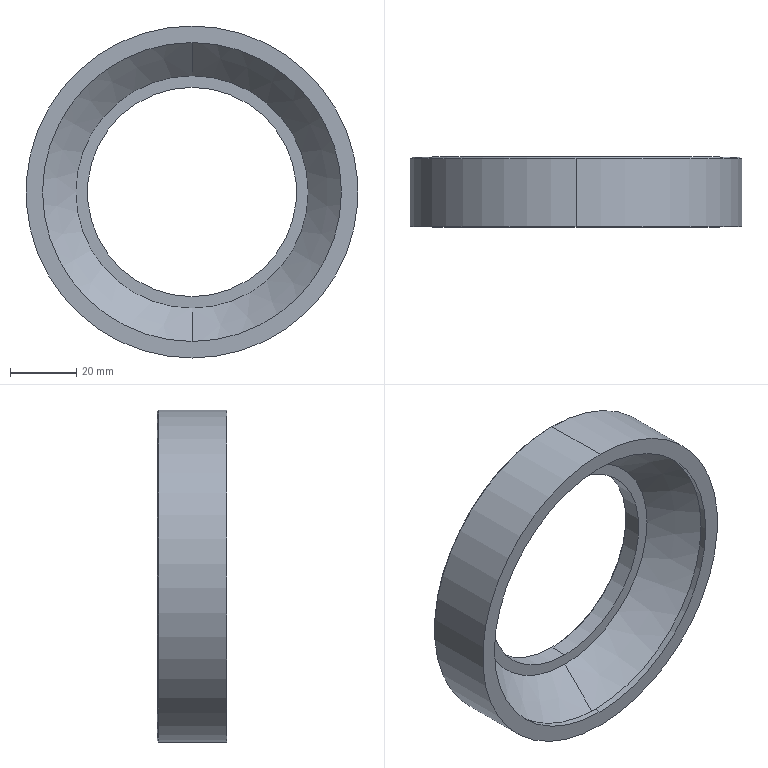Part | STEP file | WLDR-LA100-W light source | 1 solid | 34 faces | box 100 x 21 x 100 mm | volume 62526 mm3 | cylinder 16 | cone 14 | plane 4 | commonest cylinder face diameters 2.5 x8 63 x2 90 x2 94 x2 100 x2